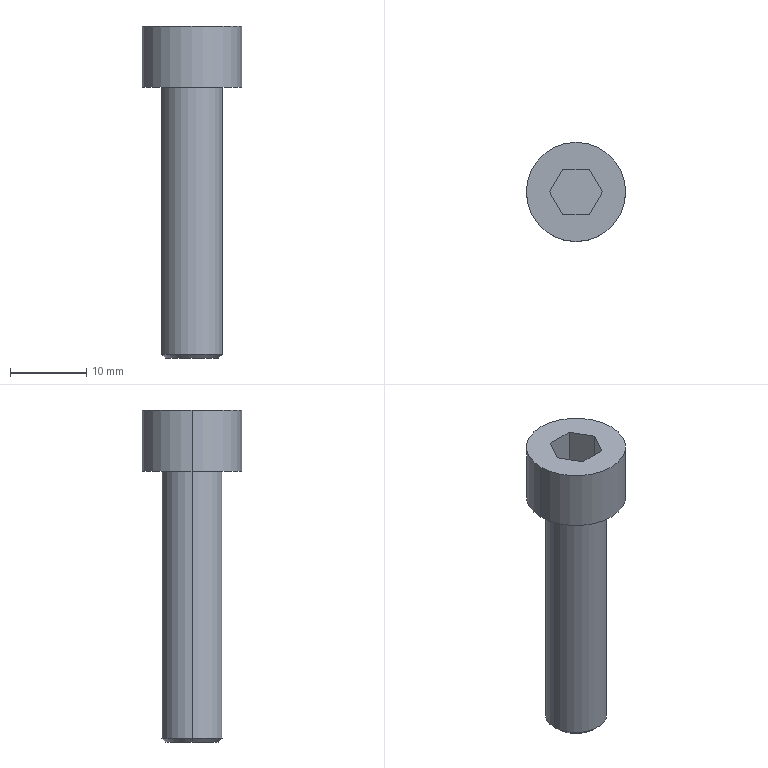Part | Creo | 1 solid | 16 faces | box 13 x 13 x 43.5 mm | volume 2679 mm3 | plane 10 | cylinder 4 | cone 2 | commonest cylinder face diameters 8 x2 13 x2
STEP:
#1=CARTESIAN_POINT('',(0.,0.,0.));
#2=DIRECTION('',(0.,0.,1.));
#3=DIRECTION('',(1.,0.,0.));
#4=AXIS2_PLACEMENT_3D('',#1,#2,#3);
#5=CARTESIAN_POINT('',(340.101,-74.745,-160.953));
#6=VERTEX_POINT('',#5);
#7=CARTESIAN_POINT('',(348.101,-74.745,-160.953));
#8=VERTEX_POINT('',#7);
#9=CARTESIAN_POINT('',(344.101,-74.745,-160.953));
#10=DIRECTION('',(0.,0.,-1.));
#11=DIRECTION('',(-1.,0.,0.));
#12=AXIS2_PLACEMENT_3D('',#9,#10,#11);
#13=CIRCLE('',#12,4.);
#14=EDGE_CURVE('',#6,#8,#13,.T.);
#15=ORIENTED_EDGE('',*,*,#14,.T.);
#16=CARTESIAN_POINT('',(348.101,-74.745,-125.96));
#17=VERTEX_POINT('',#16);
#18=CARTESIAN_POINT('',(348.101,-74.745,-125.96));
#19=DIRECTION('',(0.,0.,-1.));
#20=VECTOR('',#19,34.993);
#21=LINE('',#18,#20);
#22=EDGE_CURVE('',#17,#8,#21,.T.);
#23=ORIENTED_EDGE('',*,*,#22,.F.);
#24=CARTESIAN_POINT('',(340.101,-74.745,-125.96));
#25=VERTEX_POINT('',#24);
#26=CARTESIAN_POINT('',(344.101,-74.745,-125.96));
#27=DIRECTION('',(0.,0.,1.));
#28=DIRECTION('',(1.,0.,0.));
#29=AXIS2_PLACEMENT_3D('',#26,#27,#28);
#30=CIRCLE('',#29,4.);
#31=EDGE_CURVE('',#17,#25,#30,.T.);
#32=ORIENTED_EDGE('',*,*,#31,.T.);
#33=CARTESIAN_POINT('',(340.101,-74.745,-125.96));
#34=DIRECTION('',(0.,0.,-1.));
#35=VECTOR('',#34,34.993);
#36=LINE('',#33,#35);
#37=EDGE_CURVE('',#25,#6,#36,.T.);
#38=ORIENTED_EDGE('',*,*,#37,.T.);
#39=EDGE_LOOP('',(#15,#23,#32,#38));
#40=FACE_OUTER_BOUND('',#39,.F.);
#41=CARTESIAN_POINT('',(344.101,-74.745,-125.96));
#42=DIRECTION('',(0.,0.,-1.));
#43=DIRECTION('',(-1.,0.,0.));
#44=AXIS2_PLACEMENT_3D('',#41,#42,#43);
#45=CYLINDRICAL_SURFACE('',#44,4.);
#46=ADVANCED_FACE('',(#40),#45,.T.);
#47=CARTESIAN_POINT('',(340.608,-74.745,-161.46));
#48=VERTEX_POINT('',#47);
#49=CARTESIAN_POINT('',(347.593,-74.745,-161.46));
#50=VERTEX_POINT('',#49);
#51=CARTESIAN_POINT('',(344.101,-74.745,-161.46));
#52=DIRECTION('',(0.,0.,-1.));
#53=DIRECTION('',(-1.,0.,0.));
#54=AXIS2_PLACEMENT_3D('',#51,#52,#53);
#55=CIRCLE('',#54,3.493);
#56=EDGE_CURVE('',#48,#50,#55,.T.);
#57=ORIENTED_EDGE('',*,*,#56,.T.);
#58=CARTESIAN_POINT('',(347.593,-74.745,-161.46));
#59=DIRECTION('',(0.7071,0.,0.7071));
#60=VECTOR('',#59,0.7176);
#61=LINE('',#58,#60);
#62=EDGE_CURVE('',#50,#8,#61,.T.);
#63=ORIENTED_EDGE('',*,*,#62,.T.);
#64=ORIENTED_EDGE('',*,*,#14,.F.);
#65=CARTESIAN_POINT('',(340.608,-74.745,-161.46));
#66=DIRECTION('',(-0.7071,0.,0.7071));
#67=VECTOR('',#66,0.7176);
#68=LINE('',#65,#67);
#69=EDGE_CURVE('',#48,#6,#68,.T.);
#70=ORIENTED_EDGE('',*,*,#69,.F.);
#71=EDGE_LOOP('',(#57,#63,#64,#70));
#72=FACE_OUTER_BOUND('',#71,.F.);
#73=CARTESIAN_POINT('',(344.101,-74.745,-161.206));
#74=DIRECTION('',(0.,0.,1.));
#75=DIRECTION('',(1.,0.,0.));
#76=AXIS2_PLACEMENT_3D('',#73,#74,#75);
#77=CONICAL_SURFACE('',#76,3.746,45.);
#78=ADVANCED_FACE('',(#72),#77,.T.);
#79=ORIENTED_EDGE('',*,*,#56,.F.);
#80=CARTESIAN_POINT('',(344.101,-74.745,-161.46));
#81=DIRECTION('',(0.,0.,-1.));
#82=DIRECTION('',(1.,0.,0.));
#83=AXIS2_PLACEMENT_3D('',#80,#81,#82);
#84=CIRCLE('',#83,3.493);
#85=EDGE_CURVE('',#50,#48,#84,.T.);
#86=ORIENTED_EDGE('',*,*,#85,.F.);
#87=EDGE_LOOP('',(#79,#86));
#88=FACE_OUTER_BOUND('',#87,.F.);
#89=CARTESIAN_POINT('',(344.101,-74.745,-161.46));
#90=DIRECTION('',(0.,0.,1.));
#91=DIRECTION('',(1.,0.,0.));
#92=AXIS2_PLACEMENT_3D('',#89,#90,#91);
#93=PLANE('',#92);
#94=ADVANCED_FACE('',(#88),#93,.F.);
#95=ORIENTED_EDGE('',*,*,#85,.T.);
#96=ORIENTED_EDGE('',*,*,#69,.T.);
#97=CARTESIAN_POINT('',(344.101,-74.745,-160.953));
#98=DIRECTION('',(0.,0.,-1.));
#99=DIRECTION('',(1.,0.,0.));
#100=AXIS2_PLACEMENT_3D('',#97,#98,#99);
#101=CIRCLE('',#100,4.);
#102=EDGE_CURVE('',#8,#6,#101,.T.);
#103=ORIENTED_EDGE('',*,*,#102,.F.);
#104=ORIENTED_EDGE('',*,*,#62,.F.);
#105=EDGE_LOOP('',(#95,#96,#103,#104));
#106=FACE_OUTER_BOUND('',#105,.F.);
#107=CARTESIAN_POINT('',(344.101,-74.745,-161.206));
#108=DIRECTION('',(0.,0.,1.));
#109=DIRECTION('',(1.,0.,0.));
#110=AXIS2_PLACEMENT_3D('',#107,#108,#109);
#111=CONICAL_SURFACE('',#110,3.746,45.);
#112=ADVANCED_FACE('',(#106),#111,.T.);
#113=ORIENTED_EDGE('',*,*,#102,.T.);
#114=ORIENTED_EDGE('',*,*,#37,.F.);
#115=CARTESIAN_POINT('',(344.101,-74.745,-125.96));
#116=DIRECTION('',(0.,0.,1.));
#117=DIRECTION('',(-1.,0.,0.));
#118=AXIS2_PLACEMENT_3D('',#115,#116,#117);
#119=CIRCLE('',#118,4.);
#120=EDGE_CURVE('',#25,#17,#119,.T.);
#121=ORIENTED_EDGE('',*,*,#120,.T.);
#122=ORIENTED_EDGE('',*,*,#22,.T.);
#123=EDGE_LOOP('',(#113,#114,#121,#122));
#124=FACE_OUTER_BOUND('',#123,.F.);
#125=CARTESIAN_POINT('',(344.101,-74.745,-125.96));
#126=DIRECTION('',(0.,0.,-1.));
#127=DIRECTION('',(-1.,0.,0.));
#128=AXIS2_PLACEMENT_3D('',#125,#126,#127);
#129=CYLINDRICAL_SURFACE('',#128,4.);
#130=ADVANCED_FACE('',(#124),#129,.T.);
#131=CARTESIAN_POINT('',(337.601,-74.745,-125.96));
#132=VERTEX_POINT('',#131);
#133=CARTESIAN_POINT('',(350.601,-74.745,-125.96));
#134=VERTEX_POINT('',#133);
#135=CARTESIAN_POINT('',(344.101,-74.745,-125.96));
#136=DIRECTION('',(0.,0.,-1.));
#137=DIRECTION('',(-1.,0.,0.));
#138=AXIS2_PLACEMENT_3D('',#135,#136,#137);
#139=CIRCLE('',#138,6.5);
#140=EDGE_CURVE('',#132,#134,#139,.T.);
#141=ORIENTED_EDGE('',*,*,#140,.F.);
#142=CARTESIAN_POINT('',(344.101,-74.745,-125.96));
#143=DIRECTION('',(0.,0.,-1.));
#144=DIRECTION('',(1.,0.,0.));
#145=AXIS2_PLACEMENT_3D('',#142,#143,#144);
#146=CIRCLE('',#145,6.5);
#147=EDGE_CURVE('',#134,#132,#146,.T.);
#148=ORIENTED_EDGE('',*,*,#147,.F.);
#149=EDGE_LOOP('',(#141,#148));
#150=FACE_OUTER_BOUND('',#149,.F.);
#151=ORIENTED_EDGE('',*,*,#120,.F.);
#152=ORIENTED_EDGE('',*,*,#31,.F.);
#153=EDGE_LOOP('',(#151,#152));
#154=FACE_BOUND('',#153,.F.);
#155=CARTESIAN_POINT('',(344.101,-74.745,-125.96));
#156=DIRECTION('',(0.,0.,-1.));
#157=DIRECTION('',(-1.,0.,0.));
#158=AXIS2_PLACEMENT_3D('',#155,#156,#157);
#159=PLANE('',#158);
#160=ADVANCED_FACE('',(#150,#154),#159,.T.);
#161=CARTESIAN_POINT('',(350.601,-74.745,-117.96));
#162=VERTEX_POINT('',#161);
#163=CARTESIAN_POINT('',(337.601,-74.745,-117.96));
#164=VERTEX_POINT('',#163);
#165=CARTESIAN_POINT('',(344.101,-74.745,-117.96));
#166=DIRECTION('',(0.,0.,1.));
#167=DIRECTION('',(1.,0.,0.));
#168=AXIS2_PLACEMENT_3D('',#165,#166,#167);
#169=CIRCLE('',#168,6.5);
#170=EDGE_CURVE('',#162,#164,#169,.T.);
#171=ORIENTED_EDGE('',*,*,#170,.T.);
#172=CARTESIAN_POINT('',(337.601,-74.745,-125.96));
#173=DIRECTION('',(0.,0.,1.));
#174=VECTOR('',#173,8.);
#175=LINE('',#172,#174);
#176=EDGE_CURVE('',#132,#164,#175,.T.);
#177=ORIENTED_EDGE('',*,*,#176,.F.);
#178=ORIENTED_EDGE('',*,*,#140,.T.);
#179=CARTESIAN_POINT('',(350.601,-74.745,-125.96));
#180=DIRECTION('',(0.,0.,1.));
#181=VECTOR('',#180,8.);
#182=LINE('',#179,#181);
#183=EDGE_CURVE('',#134,#162,#182,.T.);
#184=ORIENTED_EDGE('',*,*,#183,.T.);
#185=EDGE_LOOP('',(#171,#177,#178,#184));
#186=FACE_OUTER_BOUND('',#185,.F.);
#187=CARTESIAN_POINT('',(344.101,-74.745,-125.96));
#188=DIRECTION('',(0.,0.,1.));
#189=DIRECTION('',(1.,0.,0.));
#190=AXIS2_PLACEMENT_3D('',#187,#188,#189);
#191=CYLINDRICAL_SURFACE('',#190,6.5);
#192=ADVANCED_FACE('',(#186),#191,.T.);
#193=CARTESIAN_POINT('',(344.101,-74.745,-117.96));
#194=DIRECTION('',(0.,0.,1.));
#195=DIRECTION('',(-1.,0.,0.));
#196=AXIS2_PLACEMENT_3D('',#193,#194,#195);
#197=CIRCLE('',#196,6.5);
#198=EDGE_CURVE('',#164,#162,#197,.T.);
#199=ORIENTED_EDGE('',*,*,#198,.F.);
#200=ORIENTED_EDGE('',*,*,#170,.F.);
#201=EDGE_LOOP('',(#199,#200));
#202=FACE_OUTER_BOUND('',#201,.F.);
#203=CARTESIAN_POINT('',(342.369,-71.745,-117.96));
#204=VERTEX_POINT('',#203);
#205=CARTESIAN_POINT('',(345.833,-71.745,-117.96));
#206=VERTEX_POINT('',#205);
#207=CARTESIAN_POINT('',(342.369,-71.745,-117.96));
#208=DIRECTION('',(1.,0.,0.));
#209=VECTOR('',#208,3.464);
#210=LINE('',#207,#209);
#211=EDGE_CURVE('',#204,#206,#210,.T.);
#212=ORIENTED_EDGE('',*,*,#211,.F.);
#213=CARTESIAN_POINT('',(340.637,-74.745,-117.96));
#214=VERTEX_POINT('',#213);
#215=CARTESIAN_POINT('',(340.637,-74.745,-117.96));
#216=DIRECTION('',(0.5,0.866,0.));
#217=VECTOR('',#216,3.464);
#218=LINE('',#215,#217);
#219=EDGE_CURVE('',#214,#204,#218,.T.);
#220=ORIENTED_EDGE('',*,*,#219,.F.);
#221=CARTESIAN_POINT('',(342.369,-77.745,-117.96));
#222=VERTEX_POINT('',#221);
#223=CARTESIAN_POINT('',(342.369,-77.745,-117.96));
#224=DIRECTION('',(-0.5,0.866,0.));
#225=VECTOR('',#224,3.464);
#226=LINE('',#223,#225);
#227=EDGE_CURVE('',#222,#214,#226,.T.);
#228=ORIENTED_EDGE('',*,*,#227,.F.);
#229=CARTESIAN_POINT('',(345.833,-77.745,-117.96));
#230=VERTEX_POINT('',#229);
#231=CARTESIAN_POINT('',(345.833,-77.745,-117.96));
#232=DIRECTION('',(-1.,0.,0.));
#233=VECTOR('',#232,3.464);
#234=LINE('',#231,#233);
#235=EDGE_CURVE('',#230,#222,#234,.T.);
#236=ORIENTED_EDGE('',*,*,#235,.F.);
#237=CARTESIAN_POINT('',(347.565,-74.745,-117.96));
#238=VERTEX_POINT('',#237);
#239=CARTESIAN_POINT('',(347.565,-74.745,-117.96));
#240=DIRECTION('',(-0.5,-0.866,0.));
#241=VECTOR('',#240,3.464);
#242=LINE('',#239,#241);
#243=EDGE_CURVE('',#238,#230,#242,.T.);
#244=ORIENTED_EDGE('',*,*,#243,.F.);
#245=CARTESIAN_POINT('',(345.833,-71.745,-117.96));
#246=DIRECTION('',(0.5,-0.866,0.));
#247=VECTOR('',#246,3.464);
#248=LINE('',#245,#247);
#249=EDGE_CURVE('',#206,#238,#248,.T.);
#250=ORIENTED_EDGE('',*,*,#249,.F.);
#251=EDGE_LOOP('',(#212,#220,#228,#236,#244,#250));
#252=FACE_BOUND('',#251,.F.);
#253=CARTESIAN_POINT('',(344.101,-74.745,-117.96));
#254=DIRECTION('',(0.,0.,1.));
#255=DIRECTION('',(1.,0.,0.));
#256=AXIS2_PLACEMENT_3D('',#253,#254,#255);
#257=PLANE('',#256);
#258=ADVANCED_FACE('',(#202,#252),#257,.T.);
#259=ORIENTED_EDGE('',*,*,#211,.T.);
#260=CARTESIAN_POINT('',(345.833,-71.745,-123.24));
#261=VERTEX_POINT('',#260);
#262=CARTESIAN_POINT('',(345.833,-71.745,-117.96));
#263=DIRECTION('',(0.,0.,-1.));
#264=VECTOR('',#263,5.28);
#265=LINE('',#262,#264);
#266=EDGE_CURVE('',#206,#261,#265,.T.);
#267=ORIENTED_EDGE('',*,*,#266,.T.);
#268=CARTESIAN_POINT('',(342.369,-71.745,-123.24));
#269=VERTEX_POINT('',#268);
#270=CARTESIAN_POINT('',(342.369,-71.745,-123.24));
#271=DIRECTION('',(1.,0.,0.));
#272=VECTOR('',#271,3.464);
#273=LINE('',#270,#272);
#274=EDGE_CURVE('',#269,#261,#273,.T.);
#275=ORIENTED_EDGE('',*,*,#274,.F.);
#276=CARTESIAN_POINT('',(342.369,-71.745,-117.96));
#277=DIRECTION('',(0.,0.,-1.));
#278=VECTOR('',#277,5.28);
#279=LINE('',#276,#278);
#280=EDGE_CURVE('',#204,#269,#279,.T.);
#281=ORIENTED_EDGE('',*,*,#280,.F.);
#282=EDGE_LOOP('',(#259,#267,#275,#281));
#283=FACE_OUTER_BOUND('',#282,.F.);
#284=CARTESIAN_POINT('',(345.833,-71.745,-123.24));
#285=DIRECTION('',(0.,1.,0.));
#286=DIRECTION('',(0.,0.,1.));
#287=AXIS2_PLACEMENT_3D('',#284,#285,#286);
#288=PLANE('',#287);
#289=ADVANCED_FACE('',(#283),#288,.F.);
#290=ORIENTED_EDGE('',*,*,#249,.T.);
#291=CARTESIAN_POINT('',(347.565,-74.745,-123.24));
#292=VERTEX_POINT('',#291);
#293=CARTESIAN_POINT('',(347.565,-74.745,-117.96));
#294=DIRECTION('',(0.,0.,-1.));
#295=VECTOR('',#294,5.28);
#296=LINE('',#293,#295);
#297=EDGE_CURVE('',#238,#292,#296,.T.);
#298=ORIENTED_EDGE('',*,*,#297,.T.);
#299=CARTESIAN_POINT('',(347.565,-74.745,-123.24));
#300=DIRECTION('',(-0.5,0.866,0.));
#301=VECTOR('',#300,3.464);
#302=LINE('',#299,#301);
#303=EDGE_CURVE('',#292,#261,#302,.T.);
#304=ORIENTED_EDGE('',*,*,#303,.T.);
#305=ORIENTED_EDGE('',*,*,#266,.F.);
#306=EDGE_LOOP('',(#290,#298,#304,#305));
#307=FACE_OUTER_BOUND('',#306,.F.);
#308=CARTESIAN_POINT('',(347.565,-74.745,-123.24));
#309=DIRECTION('',(0.866,0.5,0.));
#310=DIRECTION('',(-0.5,0.866,0.));
#311=AXIS2_PLACEMENT_3D('',#308,#309,#310);
#312=PLANE('',#311);
#313=ADVANCED_FACE('',(#307),#312,.F.);
#314=ORIENTED_EDGE('',*,*,#243,.T.);
#315=CARTESIAN_POINT('',(345.833,-77.745,-123.24));
#316=VERTEX_POINT('',#315);
#317=CARTESIAN_POINT('',(345.833,-77.745,-117.96));
#318=DIRECTION('',(0.,0.,-1.));
#319=VECTOR('',#318,5.28);
#320=LINE('',#317,#319);
#321=EDGE_CURVE('',#230,#316,#320,.T.);
#322=ORIENTED_EDGE('',*,*,#321,.T.);
#323=CARTESIAN_POINT('',(345.833,-77.745,-123.24));
#324=DIRECTION('',(0.5,0.866,0.));
#325=VECTOR('',#324,3.464);
#326=LINE('',#323,#325);
#327=EDGE_CURVE('',#316,#292,#326,.T.);
#328=ORIENTED_EDGE('',*,*,#327,.T.);
#329=ORIENTED_EDGE('',*,*,#297,.F.);
#330=EDGE_LOOP('',(#314,#322,#328,#329));
#331=FACE_OUTER_BOUND('',#330,.F.);
#332=CARTESIAN_POINT('',(345.833,-77.745,-123.24));
#333=DIRECTION('',(0.866,-0.5,0.));
#334=DIRECTION('',(0.5,0.866,0.));
#335=AXIS2_PLACEMENT_3D('',#332,#333,#334);
#336=PLANE('',#335);
#337=ADVANCED_FACE('',(#331),#336,.F.);
#338=ORIENTED_EDGE('',*,*,#235,.T.);
#339=CARTESIAN_POINT('',(342.369,-77.745,-123.24));
#340=VERTEX_POINT('',#339);
#341=CARTESIAN_POINT('',(342.369,-77.745,-117.96));
#342=DIRECTION('',(0.,0.,-1.));
#343=VECTOR('',#342,5.28);
#344=LINE('',#341,#343);
#345=EDGE_CURVE('',#222,#340,#344,.T.);
#346=ORIENTED_EDGE('',*,*,#345,.T.);
#347=CARTESIAN_POINT('',(345.833,-77.745,-123.24));
#348=DIRECTION('',(-1.,0.,0.));
#349=VECTOR('',#348,3.464);
#350=LINE('',#347,#349);
#351=EDGE_CURVE('',#316,#340,#350,.T.);
#352=ORIENTED_EDGE('',*,*,#351,.F.);
#353=ORIENTED_EDGE('',*,*,#321,.F.);
#354=EDGE_LOOP('',(#338,#346,#352,#353));
#355=FACE_OUTER_BOUND('',#354,.F.);
#356=CARTESIAN_POINT('',(342.369,-77.745,-123.24));
#357=DIRECTION('',(0.,-1.,0.));
#358=DIRECTION('',(0.,0.,-1.));
#359=AXIS2_PLACEMENT_3D('',#356,#357,#358);
#360=PLANE('',#359);
#361=ADVANCED_FACE('',(#355),#360,.F.);
#362=ORIENTED_EDGE('',*,*,#227,.T.);
#363=CARTESIAN_POINT('',(340.637,-74.745,-123.24));
#364=VERTEX_POINT('',#363);
#365=CARTESIAN_POINT('',(340.637,-74.745,-117.96));
#366=DIRECTION('',(0.,0.,-1.));
#367=VECTOR('',#366,5.28);
#368=LINE('',#365,#367);
#369=EDGE_CURVE('',#214,#364,#368,.T.);
#370=ORIENTED_EDGE('',*,*,#369,.T.);
#371=CARTESIAN_POINT('',(340.637,-74.745,-123.24));
#372=DIRECTION('',(0.5,-0.866,0.));
#373=VECTOR('',#372,3.464);
#374=LINE('',#371,#373);
#375=EDGE_CURVE('',#364,#340,#374,.T.);
#376=ORIENTED_EDGE('',*,*,#375,.T.);
#377=ORIENTED_EDGE('',*,*,#345,.F.);
#378=EDGE_LOOP('',(#362,#370,#376,#377));
#379=FACE_OUTER_BOUND('',#378,.F.);
#380=CARTESIAN_POINT('',(340.637,-74.745,-123.24));
#381=DIRECTION('',(-0.866,-0.5,0.));
#382=DIRECTION('',(0.5,-0.866,0.));
#383=AXIS2_PLACEMENT_3D('',#380,#381,#382);
#384=PLANE('',#383);
#385=ADVANCED_FACE('',(#379),#384,.F.);
#386=ORIENTED_EDGE('',*,*,#219,.T.);
#387=ORIENTED_EDGE('',*,*,#280,.T.);
#388=CARTESIAN_POINT('',(342.369,-71.745,-123.24));
#389=DIRECTION('',(-0.5,-0.866,0.));
#390=VECTOR('',#389,3.464);
#391=LINE('',#388,#390);
#392=EDGE_CURVE('',#269,#364,#391,.T.);
#393=ORIENTED_EDGE('',*,*,#392,.T.);
#394=ORIENTED_EDGE('',*,*,#369,.F.);
#395=EDGE_LOOP('',(#386,#387,#393,#394));
#396=FACE_OUTER_BOUND('',#395,.F.);
#397=CARTESIAN_POINT('',(342.369,-71.745,-123.24));
#398=DIRECTION('',(-0.866,0.5,0.));
#399=DIRECTION('',(-0.5,-0.866,0.));
#400=AXIS2_PLACEMENT_3D('',#397,#398,#399);
#401=PLANE('',#400);
#402=ADVANCED_FACE('',(#396),#401,.F.);
#403=ORIENTED_EDGE('',*,*,#274,.T.);
#404=ORIENTED_EDGE('',*,*,#303,.F.);
#405=ORIENTED_EDGE('',*,*,#327,.F.);
#406=ORIENTED_EDGE('',*,*,#351,.T.);
#407=ORIENTED_EDGE('',*,*,#375,.F.);
#408=ORIENTED_EDGE('',*,*,#392,.F.);
#409=EDGE_LOOP('',(#403,#404,#405,#406,#407,#408));
#410=FACE_OUTER_BOUND('',#409,.F.);
#411=CARTESIAN_POINT('',(342.369,-71.745,-123.24));
#412=DIRECTION('',(0.,0.,1.));
#413=DIRECTION('',(1.,0.,0.));
#414=AXIS2_PLACEMENT_3D('',#411,#412,#413);
#415=PLANE('',#414);
#416=ADVANCED_FACE('',(#410),#415,.T.);
#417=ORIENTED_EDGE('',*,*,#198,.T.);
#418=ORIENTED_EDGE('',*,*,#183,.F.);
#419=ORIENTED_EDGE('',*,*,#147,.T.);
#420=ORIENTED_EDGE('',*,*,#176,.T.);
#421=EDGE_LOOP('',(#417,#418,#419,#420));
#422=FACE_OUTER_BOUND('',#421,.F.);
#423=CARTESIAN_POINT('',(344.101,-74.745,-125.96));
#424=DIRECTION('',(0.,0.,1.));
#425=DIRECTION('',(1.,0.,0.));
#426=AXIS2_PLACEMENT_3D('',#423,#424,#425);
#427=CYLINDRICAL_SURFACE('',#426,6.5);
#428=ADVANCED_FACE('',(#422),#427,.T.);
#429=CLOSED_SHELL('',(#46,#78,#94,#112,#130,#160,#192,#258,#289,#313,#337,#361,#385,#402,#416,#428));
#430=MANIFOLD_SOLID_BREP('',#429);
#431=(LENGTH_UNIT()NAMED_UNIT(*)SI_UNIT(.MILLI.,.METRE.));
#432=UNCERTAINTY_MEASURE_WITH_UNIT(LENGTH_MEASURE(0.004722),#431,'','');
#433=(NAMED_UNIT(*)PLANE_ANGLE_UNIT()SI_UNIT($,.RADIAN.));
#434=PLANE_ANGLE_MEASURE_WITH_UNIT(PLANE_ANGLE_MEASURE(0.01745),#433);
#435=(CONVERSION_BASED_UNIT('DEGREE',#434)NAMED_UNIT(*)PLANE_ANGLE_UNIT());
#436=(NAMED_UNIT(*)SI_UNIT($,.STERADIAN.)SOLID_ANGLE_UNIT());
#437=(GEOMETRIC_REPRESENTATION_CONTEXT(3)GLOBAL_UNCERTAINTY_ASSIGNED_CONTEXT((#432))GLOBAL_UNIT_ASSIGNED_CONTEXT((#431,#435,#436))REPRESENTATION_CONTEXT('',''));
#438=ADVANCED_BREP_SHAPE_REPRESENTATION('',(#4,#430),#437);